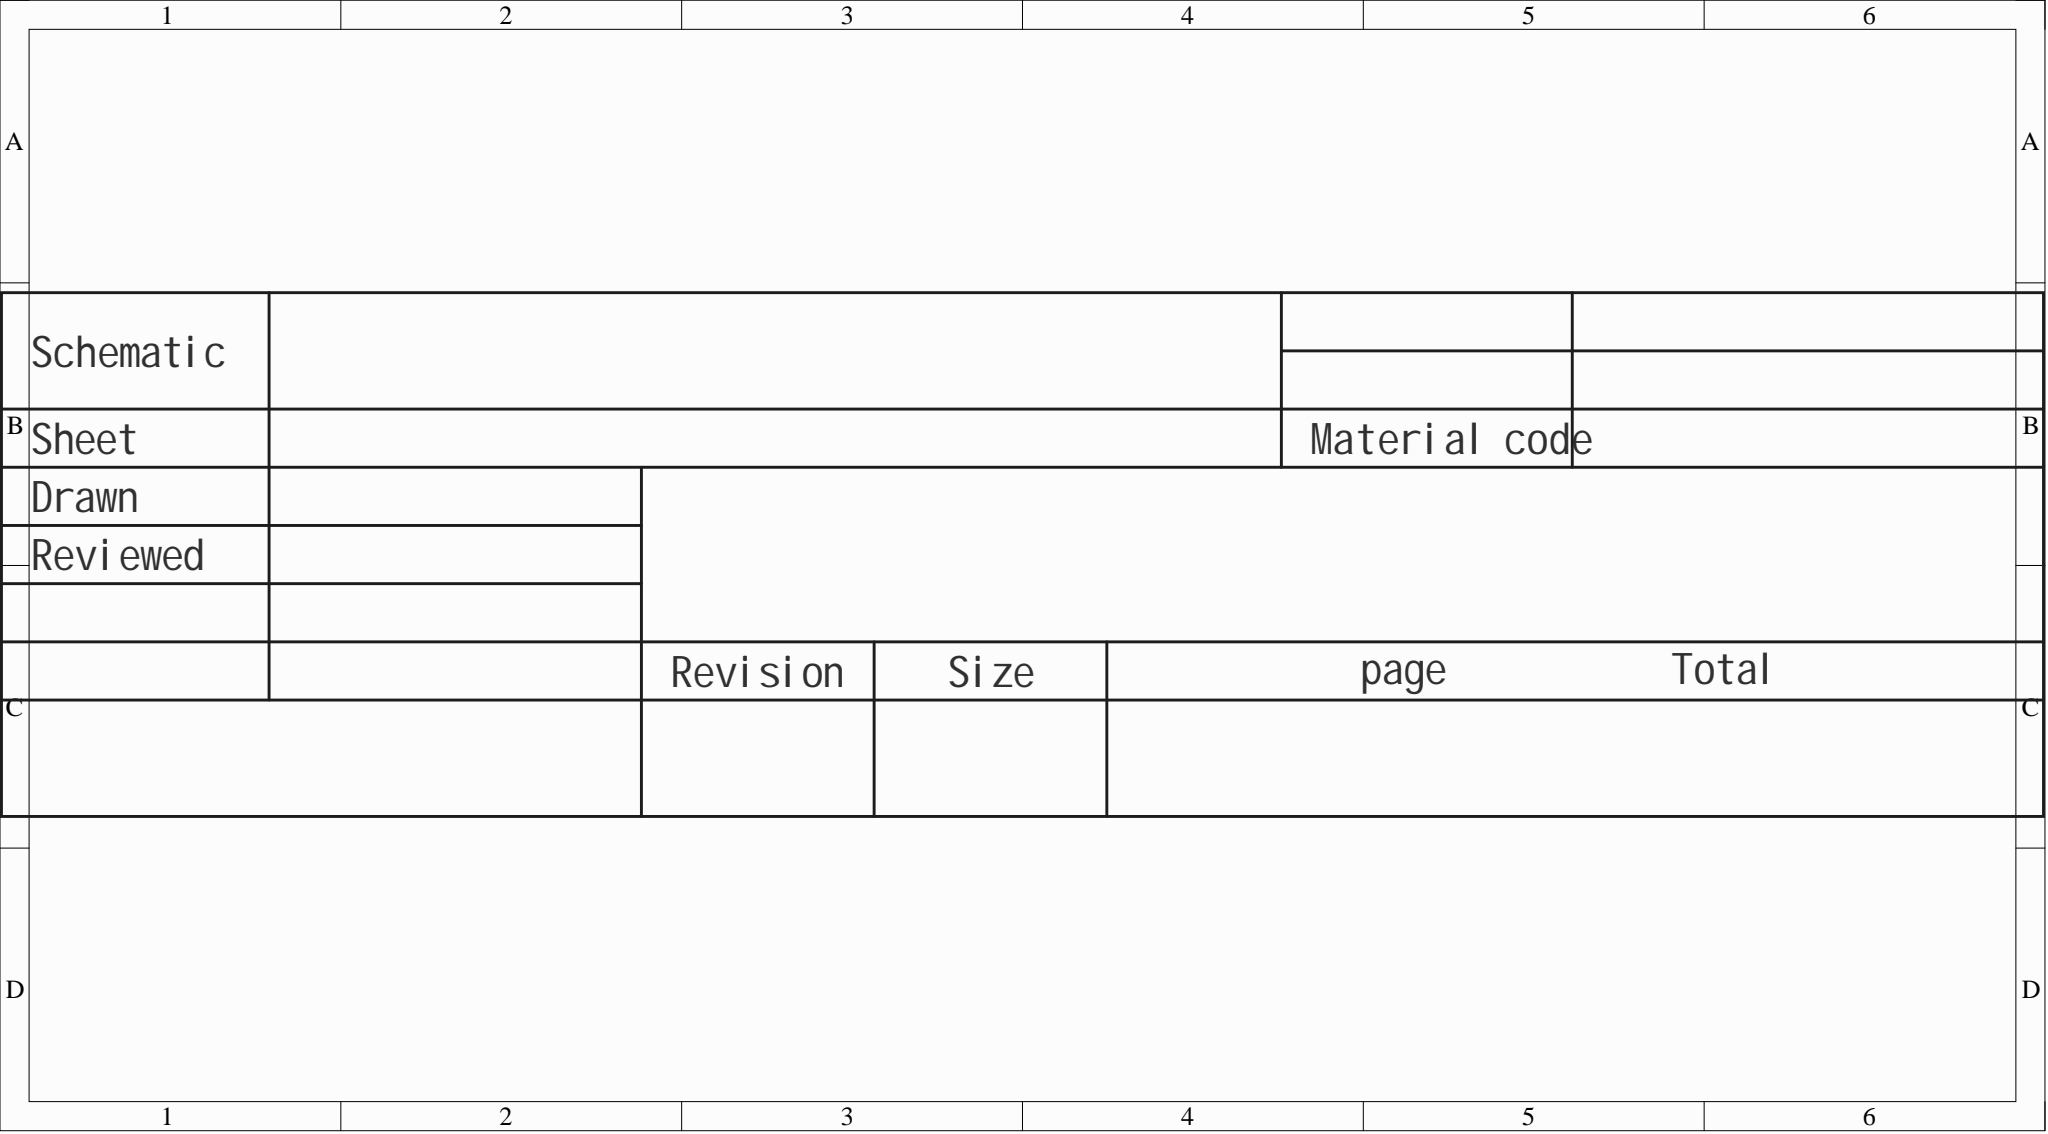Circuit board | Altium Designer | 30 parts | 36 nets
Bill of materials:
Comment,Description,Designator,Footprint,LibRef,Quantity
"buzzer-12X9","","BUZZER1","BUZ-TH_BD12.0-P7.60-D0.6-FD","buzzer-12X9","1"
"10uf","","C1","C0805","CAP_0805","1"
"30pf","","C2, C3","C0805","CAP_0805","2"
"","","H1","HDR-TH_9P-P2.54-V-F-1","HDR-F_2.54_1x9P","1"
"","","H2","HDR-TH_6P-P2.54-V-M-1","HDR-M_2.54_1x6P","1"
"","","H3, H4","HDR-TH_4P-P2.54-V-M","HDR-M_2.54_1x4P","2"
"","","H5","HDR-TH_2P-P2.54-V-M-1","HDR-M_2.54_1x2P","1"
"LMB162ADC","16x2 character LCD module","LCD1","LCD1602","LMB162ADC","1"
"","","LEDG1, LEDG2, LEDR1","LED_0805","LED_0805-R","3"
"2N3906S-RTK/PS","","Q1","SOT-23-3_L2.9-W1.3-P1.90-LS2.4-TR","2N3906S-RTK/PS","1"
"10K","","R1, R2","R0805","Res_0805","2"
"1K","","R3","R0805","Res_0805","1"
"220","","R4, R5, R7","R0805","Res_0805","3"
"2.2K","","R6","R0805","Res_0805","1"
"Tact switch 3*6*2.5","","SW1, SW2, SW3, SW4","SW-SMD_L6.0-W3.6-LS8.0","轻触按键3*6*2.5","4"
"DSWB04LHGET","Type: flat toggle, raised; circuit: SPST; switch positions: 4; lifetime: -; color: red;","SW5","SW-TH_DSWB04LHGET","DSWB04LHGET","1"
"STC89C516RD+40I-PDIP40","CPU core: 51 series; program memory: 61KB; total RAM: 1.25KB; GPIO ports: 35; operating voltage: 3.5V~5.5V; max CPU clock: -; program memory type: FLASH;","U1","DIP-40_L52.3-W13.9-P2.54-LS15.2-BL","STC89C516RD+40I-PDIP40","1"
"11.059MHz","Frequency: 12MHz; frequency tolerance at room temperature: ±30ppm; external load capacitance: -; frequency stability (full temperature): ±50ppm;","U2","HC-49US_L11.0-W4.6-P4.88","ECS-120-S-4","1"
"SN74LS126ADR2","","U5","SOIC-14_L8.7-W3.9-P1.27-LS6.0-BL","SN74LS126ADR2","1"
"DM74LS125ASJ","Supply voltage: 4.75V~5.25V; elements: 4; bits per element: 1; sink current (IOL): 24mA; source current (IOH): 2.6mA;","U6","SOP-14_L10.2-W5.3-P1.27-LS7.8-BL","DM74LS125ASJ","1"
Netlist (Protel format):
[
BUZZER1
BUZ-TH_BD12.0-P7.60-D0.6-FD
buzzer-12X9



]
[
C1
C0805
10uf



]
[
C2
C0805
30pf



]
[
C3
C0805
30pf



]
[
H1
HDR-TH_9P-P2.54-V-F-1




]
[
H2
HDR-TH_6P-P2.54-V-M-1




]
[
H3
HDR-TH_4P-P2.54-V-M




]
[
H4
HDR-TH_4P-P2.54-V-M




]
[
H5
HDR-TH_2P-P2.54-V-M-1




]
[
LCD1
LCD1602
LMB162ADC



]
[
LEDG1
LED_0805




]
[
LEDG2
LED_0805




]
[
LEDR1
LED_0805




]
[
Q1
SOT-23-3_L2.9-W1.3-P1.90-LS2.4-TR
2N3906S-RTK/PS



]
[
R1
R0805
10K



]
[
R2
R0805
10K



]
[
R3
R0805
1K



]
[
R4
R0805
220



]
[
R5
R0805
220



]
[
R6
R0805
2.2K



]
[
R7
R0805
220



]
[
SW1
SW-SMD_L6.0-W3.6-LS8.0
Tact switch 3*6*2.5



]
[
SW2
SW-SMD_L6.0-W3.6-LS8.0
Tact switch 3*6*2.5



]
[
SW3
SW-SMD_L6.0-W3.6-LS8.0
Tact switch 3*6*2.5



]
[
SW4
SW-SMD_L6.0-W3.6-LS8.0
Tact switch 3*6*2.5



]
[
SW5
SW-TH_DSWB04LHGET
DSWB04LHGET



]
[
U1
DIP-40_L52.3-W13.9-P2.54-LS15.2-BL
STC89C516RD+40I-PDIP40



]
[
U2
HC-49US_L11.0-W4.6-P4.88
11.0592MHz



]
[
U5
SOIC-14_L8.7-W3.9-P1.27-LS6.0-BL
SN74LS126ADR2



]
[
U6
SOP-14_L10.2-W5.3-P1.27-LS7.8-BL
DM74LS125ASJ



]
(
VCC
BUZZER1-2
C1-2
H1-1
H2-2
H3-3
H4-4
H5-2
LCD1-2
LCD1-15
R2-2
R4-2
R5-2
R7-2
SW1-2
U1-40
U5-14
U6-14
)
(
TX2
H3-2
U6-5
)
(
TX1
H2-4
U5-5
)
(
TX0
H4-2
SW5-3
SW5-4
U1-11
)
(
TX
SW5-7
SW5-8
U5-2
U6-2
)
(
RX2
H3-1
U6-3
)
(
RX1
H2-5
U5-3
)
(
RX0
H4-1
SW5-1
SW5-2
U1-10
)
(
RX
SW5-5
SW5-6
U5-6
U6-6
)
(
RS
LCD1-4
U1-24
)
(
NetU1_14
U1-14
U5-1
U5-4
U6-1
U6-4
)
(
NetSW4_1
SW4-1
U1-17
)
(
NetSW3_1
SW3-1
U1-28
)
(
NetSW2_1
SW2-1
U1-27
)
(
NetR6_1
R6-1
U1-26
)
(
NetQ1_2
Q1-2
R6-2
)
(
NetLEDR1_2
LEDR1-2
R4-1
)
(
NetLEDR1_1
LEDR1-1
U1-23
)
(
NetLEDG2_2
LEDG2-2
R7-1
)
(
NetLEDG1_2
LEDG1-2
R5-1
)
(
NetLEDG1_1
LEDG1-1
U1-21
)
(
NetLCD1_3
LCD1-3
R2-1
R3-2
)
(
NetH1_9
H1-9
LCD1-14
U1-32
)
(
NetH1_8
H1-8
LCD1-13
U1-33
)
(
NetH1_7
H1-7
LCD1-12
U1-34
)
(
NetH1_6
H1-6
LCD1-11
U1-35
)
(
NetH1_5
H1-5
LCD1-10
U1-36
)
(
NetH1_4
H1-4
LCD1-9
U1-37
)
(
NetH1_3
H1-3
LCD1-8
U1-38
)
(
NetH1_2
H1-2
LCD1-7
U1-39
)
(
NetC3_2
C3-2
U1-19
U2-2
)
(
NetC2_2
C2-2
U1-18
U2-1
)
(
NetC1_1
C1-1
R1-1
SW1-1
U1-9
)
(
NetBUZZER1_1
BUZZER1-1
Q1-1
)
(
GND
C2-1
C3-1
H2-3
H3-4
H4-3
H5-1
LCD1-1
LCD1-5
LCD1-16
LEDG2-1
Q1-3
R1-2
R3-1
SW2-2
SW3-2
SW4-2
U1-20
U5-7
U6-7
)
(
EN
LCD1-6
U1-25
)